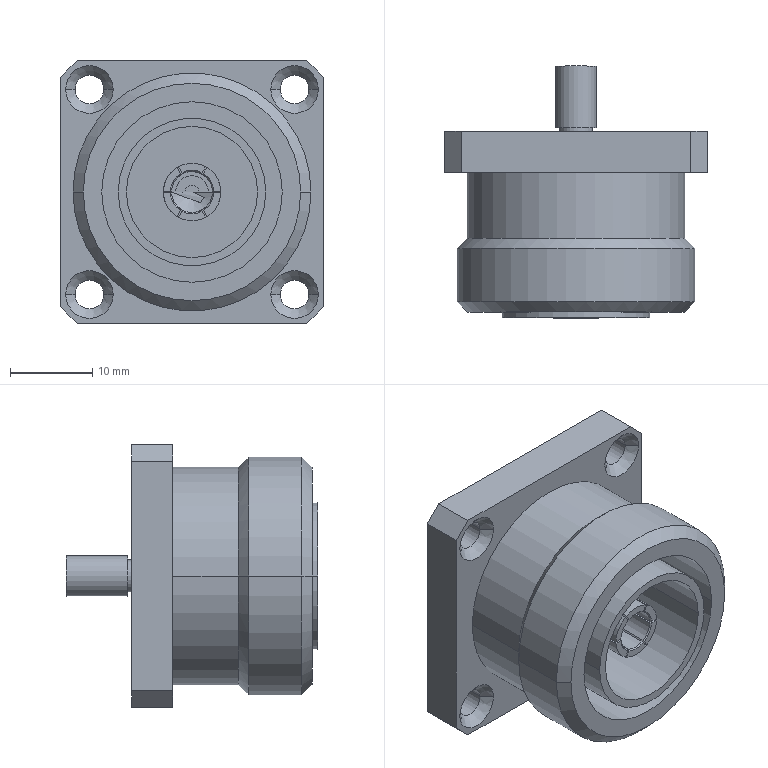Part | STEP file | 连接器 L29-KFD-9 | 2 solids | 97 faces | box 32 x 30.7 x 32 mm | volume 11064 mm3 | plane 45 | cylinder 30 | cone 22 | commonest cylinder face diameters 3.5 x8 5 x7 7 x3 16 x2 18 x2 22 x2